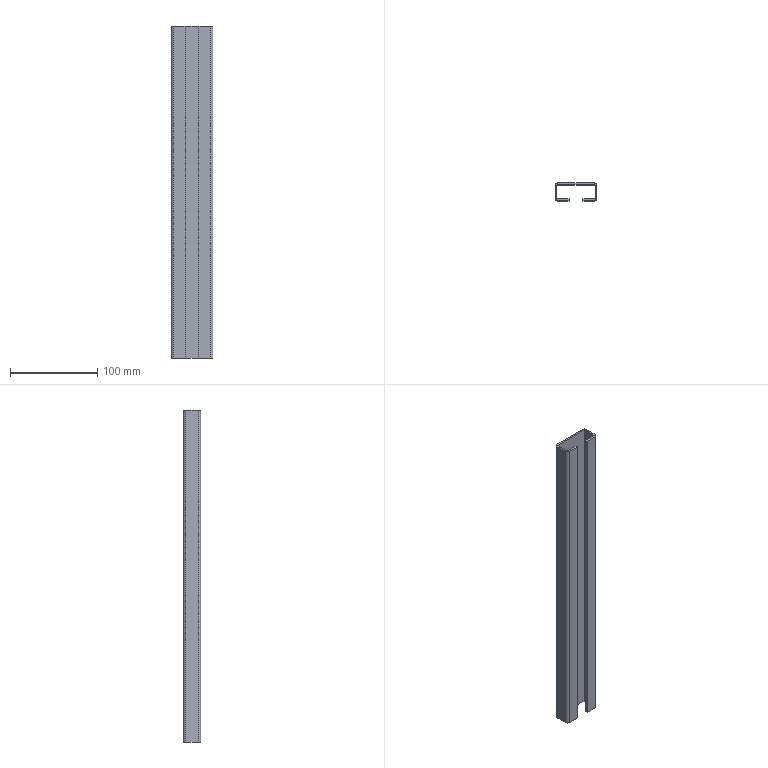Part | SolidWorks | features FlatPattern 1, SMBaseFlange 1, SheetMetal 1 | 1 solid | 38 faces | box 48 x 20 x 380 mm | volume 82510 mm3 | plane 30 | cylinder 8 | commonest cylinder face diameters 2 x4 6 x4
STEP:
#1=CARTESIAN_POINT('',(-24.,-17.,190.));
#2=VERTEX_POINT('',#1);
#3=CARTESIAN_POINT('',(-22.,-17.,190.));
#4=VERTEX_POINT('',#3);
#5=CARTESIAN_POINT('',(-24.,-17.,190.));
#6=DIRECTION('',(1.,0.,0.));
#7=VECTOR('',#6,1000.);
#8=LINE('',#5,#7);
#9=EDGE_CURVE('',#2,#4,#8,.T.);
#10=ORIENTED_EDGE('',*,*,#9,.F.);
#11=CARTESIAN_POINT('',(-21.,-20.,190.));
#12=VERTEX_POINT('',#11);
#13=CARTESIAN_POINT('',(-21.,-17.,190.));
#14=DIRECTION('',(0.,0.,-1.));
#15=DIRECTION('',(1.,0.,0.));
#16=AXIS2_PLACEMENT_3D('',#13,#14,#15);
#17=CIRCLE('',#16,3.);
#18=EDGE_CURVE('',#12,#2,#17,.T.);
#19=ORIENTED_EDGE('',*,*,#18,.F.);
#20=CARTESIAN_POINT('',(-21.,-18.,190.));
#21=VERTEX_POINT('',#20);
#22=CARTESIAN_POINT('',(-21.,-18.,190.));
#23=DIRECTION('',(0.,-1.,0.));
#24=VECTOR('',#23,1000.);
#25=LINE('',#22,#24);
#26=EDGE_CURVE('',#21,#12,#25,.T.);
#27=ORIENTED_EDGE('',*,*,#26,.F.);
#28=CARTESIAN_POINT('',(-21.,-17.,190.));
#29=DIRECTION('',(0.,0.,-1.));
#30=DIRECTION('',(1.,0.,0.));
#31=AXIS2_PLACEMENT_3D('',#28,#29,#30);
#32=CIRCLE('',#31,1.);
#33=EDGE_CURVE('',#21,#4,#32,.T.);
#34=ORIENTED_EDGE('',*,*,#33,.T.);
#35=EDGE_LOOP('',(#10,#19,#27,#34));
#36=FACE_OUTER_BOUND('',#35,.T.);
#37=CARTESIAN_POINT('',(-24.,-17.,190.));
#38=DIRECTION('',(0.,0.,1.));
#39=DIRECTION('',(1.,0.,0.));
#40=AXIS2_PLACEMENT_3D('',#37,#38,#39);
#41=PLANE('',#40);
#42=ADVANCED_FACE('',(#36),#41,.T.);
#43=CARTESIAN_POINT('',(-24.,-3.,190.));
#44=VERTEX_POINT('',#43);
#45=CARTESIAN_POINT('',(-24.,-20.,190.));
#46=DIRECTION('',(0.,1.,0.));
#47=VECTOR('',#46,1000.);
#48=LINE('',#45,#47);
#49=EDGE_CURVE('',#2,#44,#48,.T.);
#50=ORIENTED_EDGE('',*,*,#49,.F.);
#51=ORIENTED_EDGE('',*,*,#9,.T.);
#52=CARTESIAN_POINT('',(-22.,-3.,190.));
#53=VERTEX_POINT('',#52);
#54=CARTESIAN_POINT('',(-22.,-20.,190.));
#55=DIRECTION('',(0.,1.,0.));
#56=VECTOR('',#55,1000.);
#57=LINE('',#54,#56);
#58=EDGE_CURVE('',#4,#53,#57,.T.);
#59=ORIENTED_EDGE('',*,*,#58,.T.);
#60=CARTESIAN_POINT('',(-22.,-3.,190.));
#61=DIRECTION('',(-1.,0.,0.));
#62=VECTOR('',#61,1000.);
#63=LINE('',#60,#62);
#64=EDGE_CURVE('',#53,#44,#63,.T.);
#65=ORIENTED_EDGE('',*,*,#64,.T.);
#66=EDGE_LOOP('',(#50,#51,#59,#65));
#67=FACE_OUTER_BOUND('',#66,.T.);
#68=CARTESIAN_POINT('',(-21.,-18.,190.));
#69=DIRECTION('',(0.,0.,1.));
#70=DIRECTION('',(1.,0.,0.));
#71=AXIS2_PLACEMENT_3D('',#68,#69,#70);
#72=PLANE('',#71);
#73=ADVANCED_FACE('',(#67),#72,.T.);
#74=CARTESIAN_POINT('',(-21.,-20.,-190.));
#75=VERTEX_POINT('',#74);
#76=CARTESIAN_POINT('',(-21.,-18.,-190.));
#77=VERTEX_POINT('',#76);
#78=CARTESIAN_POINT('',(-21.,-20.,-190.));
#79=DIRECTION('',(0.,1.,0.));
#80=VECTOR('',#79,1000.);
#81=LINE('',#78,#80);
#82=EDGE_CURVE('',#75,#77,#81,.T.);
#83=ORIENTED_EDGE('',*,*,#82,.F.);
#84=CARTESIAN_POINT('',(-24.,-17.,-190.));
#85=VERTEX_POINT('',#84);
#86=CARTESIAN_POINT('',(-21.,-17.,-190.));
#87=DIRECTION('',(0.,0.,-1.));
#88=DIRECTION('',(1.,0.,0.));
#89=AXIS2_PLACEMENT_3D('',#86,#87,#88);
#90=CIRCLE('',#89,3.);
#91=EDGE_CURVE('',#75,#85,#90,.T.);
#92=ORIENTED_EDGE('',*,*,#91,.T.);
#93=CARTESIAN_POINT('',(-22.,-17.,-190.));
#94=VERTEX_POINT('',#93);
#95=CARTESIAN_POINT('',(-22.,-17.,-190.));
#96=DIRECTION('',(-1.,0.,0.));
#97=VECTOR('',#96,1000.);
#98=LINE('',#95,#97);
#99=EDGE_CURVE('',#94,#85,#98,.T.);
#100=ORIENTED_EDGE('',*,*,#99,.F.);
#101=CARTESIAN_POINT('',(-21.,-17.,-190.));
#102=DIRECTION('',(0.,0.,-1.));
#103=DIRECTION('',(1.,0.,0.));
#104=AXIS2_PLACEMENT_3D('',#101,#102,#103);
#105=CIRCLE('',#104,1.);
#106=EDGE_CURVE('',#77,#94,#105,.T.);
#107=ORIENTED_EDGE('',*,*,#106,.F.);
#108=EDGE_LOOP('',(#83,#92,#100,#107));
#109=FACE_OUTER_BOUND('',#108,.T.);
#110=CARTESIAN_POINT('',(-21.,-20.,-190.));
#111=DIRECTION('',(0.,0.,-1.));
#112=DIRECTION('',(-1.,0.,0.));
#113=AXIS2_PLACEMENT_3D('',#110,#111,#112);
#114=PLANE('',#113);
#115=ADVANCED_FACE('',(#109),#114,.T.);
#116=CARTESIAN_POINT('',(-8.,-20.,-190.));
#117=VERTEX_POINT('',#116);
#118=CARTESIAN_POINT('',(-8.,-20.,-190.));
#119=DIRECTION('',(-1.,0.,0.));
#120=VECTOR('',#119,1000.);
#121=LINE('',#118,#120);
#122=EDGE_CURVE('',#117,#75,#121,.T.);
#123=ORIENTED_EDGE('',*,*,#122,.T.);
#124=ORIENTED_EDGE('',*,*,#82,.T.);
#125=CARTESIAN_POINT('',(-8.,-18.,-190.));
#126=VERTEX_POINT('',#125);
#127=CARTESIAN_POINT('',(-8.,-18.,-190.));
#128=DIRECTION('',(-1.,0.,0.));
#129=VECTOR('',#128,1000.);
#130=LINE('',#127,#129);
#131=EDGE_CURVE('',#126,#77,#130,.T.);
#132=ORIENTED_EDGE('',*,*,#131,.F.);
#133=CARTESIAN_POINT('',(-8.,-18.,-190.));
#134=DIRECTION('',(0.,-1.,0.));
#135=VECTOR('',#134,1000.);
#136=LINE('',#133,#135);
#137=EDGE_CURVE('',#126,#117,#136,.T.);
#138=ORIENTED_EDGE('',*,*,#137,.T.);
#139=EDGE_LOOP('',(#123,#124,#132,#138));
#140=FACE_OUTER_BOUND('',#139,.T.);
#141=CARTESIAN_POINT('',(-22.,-17.,-190.));
#142=DIRECTION('',(0.,0.,-1.));
#143=DIRECTION('',(-1.,0.,0.));
#144=AXIS2_PLACEMENT_3D('',#141,#142,#143);
#145=PLANE('',#144);
#146=ADVANCED_FACE('',(#140),#145,.T.);
#147=CARTESIAN_POINT('',(-21.,0.,190.));
#148=VERTEX_POINT('',#147);
#149=CARTESIAN_POINT('',(-21.,-2.,190.));
#150=VERTEX_POINT('',#149);
#151=CARTESIAN_POINT('',(-21.,0.,190.));
#152=DIRECTION('',(0.,-1.,0.));
#153=VECTOR('',#152,1000.);
#154=LINE('',#151,#153);
#155=EDGE_CURVE('',#148,#150,#154,.T.);
#156=ORIENTED_EDGE('',*,*,#155,.F.);
#157=CARTESIAN_POINT('',(-21.,-3.,190.));
#158=DIRECTION('',(0.,0.,-1.));
#159=DIRECTION('',(1.,0.,0.));
#160=AXIS2_PLACEMENT_3D('',#157,#158,#159);
#161=CIRCLE('',#160,3.);
#162=EDGE_CURVE('',#44,#148,#161,.T.);
#163=ORIENTED_EDGE('',*,*,#162,.F.);
#164=ORIENTED_EDGE('',*,*,#64,.F.);
#165=CARTESIAN_POINT('',(-21.,-3.,190.));
#166=DIRECTION('',(0.,0.,-1.));
#167=DIRECTION('',(1.,0.,0.));
#168=AXIS2_PLACEMENT_3D('',#165,#166,#167);
#169=CIRCLE('',#168,1.);
#170=EDGE_CURVE('',#53,#150,#169,.T.);
#171=ORIENTED_EDGE('',*,*,#170,.T.);
#172=EDGE_LOOP('',(#156,#163,#164,#171));
#173=FACE_OUTER_BOUND('',#172,.T.);
#174=CARTESIAN_POINT('',(-21.,0.,190.));
#175=DIRECTION('',(0.,0.,1.));
#176=DIRECTION('',(1.,0.,0.));
#177=AXIS2_PLACEMENT_3D('',#174,#175,#176);
#178=PLANE('',#177);
#179=ADVANCED_FACE('',(#173),#178,.T.);
#180=CARTESIAN_POINT('',(21.,0.,190.));
#181=VERTEX_POINT('',#180);
#182=CARTESIAN_POINT('',(-24.,0.,190.));
#183=DIRECTION('',(1.,0.,0.));
#184=VECTOR('',#183,1000.);
#185=LINE('',#182,#184);
#186=EDGE_CURVE('',#148,#181,#185,.T.);
#187=ORIENTED_EDGE('',*,*,#186,.F.);
#188=ORIENTED_EDGE('',*,*,#155,.T.);
#189=CARTESIAN_POINT('',(21.,-2.,190.));
#190=VERTEX_POINT('',#189);
#191=CARTESIAN_POINT('',(-24.,-2.,190.));
#192=DIRECTION('',(1.,0.,0.));
#193=VECTOR('',#192,1000.);
#194=LINE('',#191,#193);
#195=EDGE_CURVE('',#150,#190,#194,.T.);
#196=ORIENTED_EDGE('',*,*,#195,.T.);
#197=CARTESIAN_POINT('',(21.,-2.,190.));
#198=DIRECTION('',(0.,1.,0.));
#199=VECTOR('',#198,1000.);
#200=LINE('',#197,#199);
#201=EDGE_CURVE('',#190,#181,#200,.T.);
#202=ORIENTED_EDGE('',*,*,#201,.T.);
#203=EDGE_LOOP('',(#187,#188,#196,#202));
#204=FACE_OUTER_BOUND('',#203,.T.);
#205=CARTESIAN_POINT('',(-22.,-3.,190.));
#206=DIRECTION('',(0.,0.,1.));
#207=DIRECTION('',(1.,0.,0.));
#208=AXIS2_PLACEMENT_3D('',#205,#206,#207);
#209=PLANE('',#208);
#210=ADVANCED_FACE('',(#204),#209,.T.);
#211=CARTESIAN_POINT('',(-24.,-3.,-190.));
#212=VERTEX_POINT('',#211);
#213=CARTESIAN_POINT('',(-22.,-3.,-190.));
#214=VERTEX_POINT('',#213);
#215=CARTESIAN_POINT('',(-24.,-3.,-190.));
#216=DIRECTION('',(1.,0.,0.));
#217=VECTOR('',#216,1000.);
#218=LINE('',#215,#217);
#219=EDGE_CURVE('',#212,#214,#218,.T.);
#220=ORIENTED_EDGE('',*,*,#219,.F.);
#221=CARTESIAN_POINT('',(-21.,0.,-190.));
#222=VERTEX_POINT('',#221);
#223=CARTESIAN_POINT('',(-21.,-3.,-190.));
#224=DIRECTION('',(0.,0.,-1.));
#225=DIRECTION('',(1.,0.,0.));
#226=AXIS2_PLACEMENT_3D('',#223,#224,#225);
#227=CIRCLE('',#226,3.);
#228=EDGE_CURVE('',#212,#222,#227,.T.);
#229=ORIENTED_EDGE('',*,*,#228,.T.);
#230=CARTESIAN_POINT('',(-21.,-2.,-190.));
#231=VERTEX_POINT('',#230);
#232=CARTESIAN_POINT('',(-21.,-2.,-190.));
#233=DIRECTION('',(0.,1.,0.));
#234=VECTOR('',#233,1000.);
#235=LINE('',#232,#234);
#236=EDGE_CURVE('',#231,#222,#235,.T.);
#237=ORIENTED_EDGE('',*,*,#236,.F.);
#238=CARTESIAN_POINT('',(-21.,-3.,-190.));
#239=DIRECTION('',(0.,0.,-1.));
#240=DIRECTION('',(1.,0.,0.));
#241=AXIS2_PLACEMENT_3D('',#238,#239,#240);
#242=CIRCLE('',#241,1.);
#243=EDGE_CURVE('',#214,#231,#242,.T.);
#244=ORIENTED_EDGE('',*,*,#243,.F.);
#245=EDGE_LOOP('',(#220,#229,#237,#244));
#246=FACE_OUTER_BOUND('',#245,.T.);
#247=CARTESIAN_POINT('',(-24.,-3.,-190.));
#248=DIRECTION('',(0.,0.,-1.));
#249=DIRECTION('',(-1.,0.,0.));
#250=AXIS2_PLACEMENT_3D('',#247,#248,#249);
#251=PLANE('',#250);
#252=ADVANCED_FACE('',(#246),#251,.T.);
#253=CARTESIAN_POINT('',(-24.,-20.,-190.));
#254=DIRECTION('',(0.,1.,0.));
#255=VECTOR('',#254,1000.);
#256=LINE('',#253,#255);
#257=EDGE_CURVE('',#85,#212,#256,.T.);
#258=ORIENTED_EDGE('',*,*,#257,.T.);
#259=ORIENTED_EDGE('',*,*,#219,.T.);
#260=CARTESIAN_POINT('',(-22.,-20.,-190.));
#261=DIRECTION('',(0.,1.,0.));
#262=VECTOR('',#261,1000.);
#263=LINE('',#260,#262);
#264=EDGE_CURVE('',#94,#214,#263,.T.);
#265=ORIENTED_EDGE('',*,*,#264,.F.);
#266=ORIENTED_EDGE('',*,*,#99,.T.);
#267=EDGE_LOOP('',(#258,#259,#265,#266));
#268=FACE_OUTER_BOUND('',#267,.T.);
#269=CARTESIAN_POINT('',(-21.,-2.,-190.));
#270=DIRECTION('',(0.,0.,-1.));
#271=DIRECTION('',(-1.,0.,0.));
#272=AXIS2_PLACEMENT_3D('',#269,#270,#271);
#273=PLANE('',#272);
#274=ADVANCED_FACE('',(#268),#273,.T.);
#275=CARTESIAN_POINT('',(24.,-3.,190.));
#276=VERTEX_POINT('',#275);
#277=CARTESIAN_POINT('',(22.,-3.,190.));
#278=VERTEX_POINT('',#277);
#279=CARTESIAN_POINT('',(24.,-3.,190.));
#280=DIRECTION('',(-1.,0.,0.));
#281=VECTOR('',#280,1000.);
#282=LINE('',#279,#281);
#283=EDGE_CURVE('',#276,#278,#282,.T.);
#284=ORIENTED_EDGE('',*,*,#283,.F.);
#285=CARTESIAN_POINT('',(21.,-3.,190.));
#286=DIRECTION('',(0.,0.,-1.));
#287=DIRECTION('',(1.,0.,0.));
#288=AXIS2_PLACEMENT_3D('',#285,#286,#287);
#289=CIRCLE('',#288,3.);
#290=EDGE_CURVE('',#181,#276,#289,.T.);
#291=ORIENTED_EDGE('',*,*,#290,.F.);
#292=ORIENTED_EDGE('',*,*,#201,.F.);
#293=CARTESIAN_POINT('',(21.,-3.,190.));
#294=DIRECTION('',(0.,0.,-1.));
#295=DIRECTION('',(1.,0.,0.));
#296=AXIS2_PLACEMENT_3D('',#293,#294,#295);
#297=CIRCLE('',#296,1.);
#298=EDGE_CURVE('',#190,#278,#297,.T.);
#299=ORIENTED_EDGE('',*,*,#298,.T.);
#300=EDGE_LOOP('',(#284,#291,#292,#299));
#301=FACE_OUTER_BOUND('',#300,.T.);
#302=CARTESIAN_POINT('',(24.,-3.,190.));
#303=DIRECTION('',(0.,0.,1.));
#304=DIRECTION('',(1.,0.,0.));
#305=AXIS2_PLACEMENT_3D('',#302,#303,#304);
#306=PLANE('',#305);
#307=ADVANCED_FACE('',(#301),#306,.T.);
#308=CARTESIAN_POINT('',(24.,-17.,190.));
#309=VERTEX_POINT('',#308);
#310=CARTESIAN_POINT('',(24.,0.,190.));
#311=DIRECTION('',(0.,-1.,0.));
#312=VECTOR('',#311,1000.);
#313=LINE('',#310,#312);
#314=EDGE_CURVE('',#276,#309,#313,.T.);
#315=ORIENTED_EDGE('',*,*,#314,.F.);
#316=ORIENTED_EDGE('',*,*,#283,.T.);
#317=CARTESIAN_POINT('',(22.,-17.,190.));
#318=VERTEX_POINT('',#317);
#319=CARTESIAN_POINT('',(22.,0.,190.));
#320=DIRECTION('',(0.,-1.,0.));
#321=VECTOR('',#320,1000.);
#322=LINE('',#319,#321);
#323=EDGE_CURVE('',#278,#318,#322,.T.);
#324=ORIENTED_EDGE('',*,*,#323,.T.);
#325=CARTESIAN_POINT('',(22.,-17.,190.));
#326=DIRECTION('',(1.,0.,0.));
#327=VECTOR('',#326,1000.);
#328=LINE('',#325,#327);
#329=EDGE_CURVE('',#318,#309,#328,.T.);
#330=ORIENTED_EDGE('',*,*,#329,.T.);
#331=EDGE_LOOP('',(#315,#316,#324,#330));
#332=FACE_OUTER_BOUND('',#331,.T.);
#333=CARTESIAN_POINT('',(21.,-2.,190.));
#334=DIRECTION('',(0.,0.,1.));
#335=DIRECTION('',(1.,0.,0.));
#336=AXIS2_PLACEMENT_3D('',#333,#334,#335);
#337=PLANE('',#336);
#338=ADVANCED_FACE('',(#332),#337,.T.);
#339=CARTESIAN_POINT('',(21.,0.,-190.));
#340=VERTEX_POINT('',#339);
#341=CARTESIAN_POINT('',(21.,-2.,-190.));
#342=VERTEX_POINT('',#341);
#343=CARTESIAN_POINT('',(21.,0.,-190.));
#344=DIRECTION('',(0.,-1.,0.));
#345=VECTOR('',#344,1000.);
#346=LINE('',#343,#345);
#347=EDGE_CURVE('',#340,#342,#346,.T.);
#348=ORIENTED_EDGE('',*,*,#347,.F.);
#349=CARTESIAN_POINT('',(24.,-3.,-190.));
#350=VERTEX_POINT('',#349);
#351=CARTESIAN_POINT('',(21.,-3.,-190.));
#352=DIRECTION('',(0.,0.,-1.));
#353=DIRECTION('',(1.,0.,0.));
#354=AXIS2_PLACEMENT_3D('',#351,#352,#353);
#355=CIRCLE('',#354,3.);
#356=EDGE_CURVE('',#340,#350,#355,.T.);
#357=ORIENTED_EDGE('',*,*,#356,.T.);
#358=CARTESIAN_POINT('',(22.,-3.,-190.));
#359=VERTEX_POINT('',#358);
#360=CARTESIAN_POINT('',(22.,-3.,-190.));
#361=DIRECTION('',(1.,0.,0.));
#362=VECTOR('',#361,1000.);
#363=LINE('',#360,#362);
#364=EDGE_CURVE('',#359,#350,#363,.T.);
#365=ORIENTED_EDGE('',*,*,#364,.F.);
#366=CARTESIAN_POINT('',(21.,-3.,-190.));
#367=DIRECTION('',(0.,0.,-1.));
#368=DIRECTION('',(1.,0.,0.));
#369=AXIS2_PLACEMENT_3D('',#366,#367,#368);
#370=CIRCLE('',#369,1.);
#371=EDGE_CURVE('',#342,#359,#370,.T.);
#372=ORIENTED_EDGE('',*,*,#371,.F.);
#373=EDGE_LOOP('',(#348,#357,#365,#372));
#374=FACE_OUTER_BOUND('',#373,.T.);
#375=CARTESIAN_POINT('',(21.,0.,-190.));
#376=DIRECTION('',(0.,0.,-1.));
#377=DIRECTION('',(-1.,0.,0.));
#378=AXIS2_PLACEMENT_3D('',#375,#376,#377);
#379=PLANE('',#378);
#380=ADVANCED_FACE('',(#374),#379,.T.);
#381=CARTESIAN_POINT('',(-24.,0.,-190.));
#382=DIRECTION('',(1.,0.,0.));
#383=VECTOR('',#382,1000.);
#384=LINE('',#381,#383);
#385=EDGE_CURVE('',#222,#340,#384,.T.);
#386=ORIENTED_EDGE('',*,*,#385,.T.);
#387=ORIENTED_EDGE('',*,*,#347,.T.);
#388=CARTESIAN_POINT('',(-24.,-2.,-190.));
#389=DIRECTION('',(1.,0.,0.));
#390=VECTOR('',#389,1000.);
#391=LINE('',#388,#390);
#392=EDGE_CURVE('',#231,#342,#391,.T.);
#393=ORIENTED_EDGE('',*,*,#392,.F.);
#394=ORIENTED_EDGE('',*,*,#236,.T.);
#395=EDGE_LOOP('',(#386,#387,#393,#394));
#396=FACE_OUTER_BOUND('',#395,.T.);
#397=CARTESIAN_POINT('',(22.,-3.,-190.));
#398=DIRECTION('',(0.,0.,-1.));
#399=DIRECTION('',(-1.,0.,0.));
#400=AXIS2_PLACEMENT_3D('',#397,#398,#399);
#401=PLANE('',#400);
#402=ADVANCED_FACE('',(#396),#401,.T.);
#403=CARTESIAN_POINT('',(21.,-20.,190.));
#404=VERTEX_POINT('',#403);
#405=CARTESIAN_POINT('',(21.,-18.,190.));
#406=VERTEX_POINT('',#405);
#407=CARTESIAN_POINT('',(21.,-20.,190.));
#408=DIRECTION('',(0.,1.,0.));
#409=VECTOR('',#408,1000.);
#410=LINE('',#407,#409);
#411=EDGE_CURVE('',#404,#406,#410,.T.);
#412=ORIENTED_EDGE('',*,*,#411,.F.);
#413=CARTESIAN_POINT('',(21.,-17.,190.));
#414=DIRECTION('',(0.,0.,-1.));
#415=DIRECTION('',(1.,0.,0.));
#416=AXIS2_PLACEMENT_3D('',#413,#414,#415);
#417=CIRCLE('',#416,3.);
#418=EDGE_CURVE('',#309,#404,#417,.T.);
#419=ORIENTED_EDGE('',*,*,#418,.F.);
#420=ORIENTED_EDGE('',*,*,#329,.F.);
#421=CARTESIAN_POINT('',(21.,-17.,190.));
#422=DIRECTION('',(0.,0.,-1.));
#423=DIRECTION('',(1.,0.,0.));
#424=AXIS2_PLACEMENT_3D('',#421,#422,#423);
#425=CIRCLE('',#424,1.);
#426=EDGE_CURVE('',#318,#406,#425,.T.);
#427=ORIENTED_EDGE('',*,*,#426,.T.);
#428=EDGE_LOOP('',(#412,#419,#420,#427));
#429=FACE_OUTER_BOUND('',#428,.T.);
#430=CARTESIAN_POINT('',(21.,-20.,190.));
#431=DIRECTION('',(0.,0.,1.));
#432=DIRECTION('',(1.,0.,0.));
#433=AXIS2_PLACEMENT_3D('',#430,#431,#432);
#434=PLANE('',#433);
#435=ADVANCED_FACE('',(#429),#434,.T.);
#436=CARTESIAN_POINT('',(8.,-20.,190.));
#437=VERTEX_POINT('',#436);
#438=CARTESIAN_POINT('',(24.,-20.,190.));
#439=DIRECTION('',(-1.,0.,0.));
#440=VECTOR('',#439,1000.);
#441=LINE('',#438,#440);
#442=EDGE_CURVE('',#404,#437,#441,.T.);
#443=ORIENTED_EDGE('',*,*,#442,.F.);
#444=ORIENTED_EDGE('',*,*,#411,.T.);
#445=CARTESIAN_POINT('',(8.,-18.,190.));
#446=VERTEX_POINT('',#445);
#447=CARTESIAN_POINT('',(24.,-18.,190.));
#448=DIRECTION('',(-1.,0.,0.));
#449=VECTOR('',#448,1000.);
#450=LINE('',#447,#449);
#451=EDGE_CURVE('',#406,#446,#450,.T.);
#452=ORIENTED_EDGE('',*,*,#451,.T.);
#453=CARTESIAN_POINT('',(8.,-20.,190.));
#454=DIRECTION('',(0.,1.,0.));
#455=VECTOR('',#454,1000.);
#456=LINE('',#453,#455);
#457=EDGE_CURVE('',#437,#446,#456,.T.);
#458=ORIENTED_EDGE('',*,*,#457,.F.);
#459=EDGE_LOOP('',(#443,#444,#452,#458));
#460=FACE_OUTER_BOUND('',#459,.T.);
#461=CARTESIAN_POINT('',(22.,-17.,190.));
#462=DIRECTION('',(0.,0.,1.));
#463=DIRECTION('',(1.,0.,0.));
#464=AXIS2_PLACEMENT_3D('',#461,#462,#463);
#465=PLANE('',#464);
#466=ADVANCED_FACE('',(#460),#465,.T.);
#467=CARTESIAN_POINT('',(24.,-17.,-190.));
#468=VERTEX_POINT('',#467);
#469=CARTESIAN_POINT('',(22.,-17.,-190.));
#470=VERTEX_POINT('',#469);
#471=CARTESIAN_POINT('',(24.,-17.,-190.));
#472=DIRECTION('',(-1.,0.,0.));
#473=VECTOR('',#472,1000.);
#474=LINE('',#471,#473);
#475=EDGE_CURVE('',#468,#470,#474,.T.);
#476=ORIENTED_EDGE('',*,*,#475,.F.);
#477=CARTESIAN_POINT('',(21.,-20.,-190.));
#478=VERTEX_POINT('',#477);
#479=CARTESIAN_POINT('',(21.,-17.,-190.));
#480=DIRECTION('',(0.,0.,-1.));
#481=DIRECTION('',(1.,0.,0.));
#482=AXIS2_PLACEMENT_3D('',#479,#480,#481);
#483=CIRCLE('',#482,3.);
#484=EDGE_CURVE('',#468,#478,#483,.T.);
#485=ORIENTED_EDGE('',*,*,#484,.T.);
#486=CARTESIAN_POINT('',(21.,-18.,-190.));
#487=VERTEX_POINT('',#486);
#488=CARTESIAN_POINT('',(21.,-18.,-190.));
#489=DIRECTION('',(0.,-1.,0.));
#490=VECTOR('',#489,1000.);
#491=LINE('',#488,#490);
#492=EDGE_CURVE('',#487,#478,#491,.T.);
#493=ORIENTED_EDGE('',*,*,#492,.F.);
#494=CARTESIAN_POINT('',(21.,-17.,-190.));
#495=DIRECTION('',(0.,0.,-1.));
#496=DIRECTION('',(1.,0.,0.));
#497=AXIS2_PLACEMENT_3D('',#494,#495,#496);
#498=CIRCLE('',#497,1.);
#499=EDGE_CURVE('',#470,#487,#498,.T.);
#500=ORIENTED_EDGE('',*,*,#499,.F.);
#501=EDGE_LOOP('',(#476,#485,#493,#500));
#502=FACE_OUTER_BOUND('',#501,.T.);
#503=CARTESIAN_POINT('',(24.,-17.,-190.));
#504=DIRECTION('',(0.,0.,-1.));
#505=DIRECTION('',(-1.,0.,0.));
#506=AXIS2_PLACEMENT_3D('',#503,#504,#505);
#507=PLANE('',#506);
#508=ADVANCED_FACE('',(#502),#507,.T.);
#509=CARTESIAN_POINT('',(24.,0.,-190.));
#510=DIRECTION('',(0.,-1.,0.));
#511=VECTOR('',#510,1000.);
#512=LINE('',#509,#511);
#513=EDGE_CURVE('',#350,#468,#512,.T.);
#514=ORIENTED_EDGE('',*,*,#513,.T.);
#515=ORIENTED_EDGE('',*,*,#475,.T.);
#516=CARTESIAN_POINT('',(22.,0.,-190.));
#517=DIRECTION('',(0.,-1.,0.));
#518=VECTOR('',#517,1000.);
#519=LINE('',#516,#518);
#520=EDGE_CURVE('',#359,#470,#519,.T.);
#521=ORIENTED_EDGE('',*,*,#520,.F.);
#522=ORIENTED_EDGE('',*,*,#364,.T.);
#523=EDGE_LOOP('',(#514,#515,#521,#522));
#524=FACE_OUTER_BOUND('',#523,.T.);
#525=CARTESIAN_POINT('',(21.,-18.,-190.));
#526=DIRECTION('',(0.,0.,-1.));
#527=DIRECTION('',(-1.,0.,0.));
#528=AXIS2_PLACEMENT_3D('',#525,#526,#527);
#529=PLANE('',#528);
#530=ADVANCED_FACE('',(#524),#529,.T.);
#531=CARTESIAN_POINT('',(8.,-18.,-190.));
#532=VERTEX_POINT('',#531);
#533=CARTESIAN_POINT('',(24.,-18.,-190.));
#534=DIRECTION('',(-1.,0.,0.));
#535=VECTOR('',#534,1000.);
#536=LINE('',#533,#535);
#537=EDGE_CURVE('',#487,#532,#536,.T.);
#538=ORIENTED_EDGE('',*,*,#537,.T.);
#539=CARTESIAN_POINT('',(8.,-18.,190.));
#540=DIRECTION('',(0.,0.,-1.));
#541=VECTOR('',#540,1000.);
#542=LINE('',#539,#541);
#543=EDGE_CURVE('',#446,#532,#542,.T.);
#544=ORIENTED_EDGE('',*,*,#543,.F.);
#545=ORIENTED_EDGE('',*,*,#451,.F.);
#546=CARTESIAN_POINT('',(21.,-18.,190.));
#547=DIRECTION('',(0.,0.,-1.));
#548=VECTOR('',#547,1000.);
#549=LINE('',#546,#548);
#550=EDGE_CURVE('',#406,#487,#549,.T.);
#551=ORIENTED_EDGE('',*,*,#550,.T.);
#552=EDGE_LOOP('',(#538,#544,#545,#551));
#553=FACE_OUTER_BOUND('',#552,.T.);
#554=CARTESIAN_POINT('',(24.,-18.,190.));
#555=DIRECTION('',(0.,-1.,0.));
#556=DIRECTION('',(1.,0.,0.));
#557=AXIS2_PLACEMENT_3D('',#554,#555,#556);
#558=PLANE('',#557);
#559=ADVANCED_FACE('',(#553),#558,.F.);
#560=CARTESIAN_POINT('',(8.,-20.,-190.));
#561=VERTEX_POINT('',#560);
#562=CARTESIAN_POINT('',(8.,-20.,-190.));
#563=DIRECTION('',(0.,1.,0.));
#564=VECTOR('',#563,1000.);
#565=LINE('',#562,#564);
#566=EDGE_CURVE('',#561,#532,#565,.T.);
#567=ORIENTED_EDGE('',*,*,#566,.F.);
#568=CARTESIAN_POINT('',(8.,-20.,190.));
#569=DIRECTION('',(0.,0.,-1.));
#570=VECTOR('',#569,1000.);
#571=LINE('',#568,#570);
#572=EDGE_CURVE('',#437,#561,#571,.T.);
#573=ORIENTED_EDGE('',*,*,#572,.F.);
#574=ORIENTED_EDGE('',*,*,#457,.T.);
#575=ORIENTED_EDGE('',*,*,#543,.T.);
#576=EDGE_LOOP('',(#567,#573,#574,#575));
#577=FACE_OUTER_BOUND('',#576,.T.);
#578=CARTESIAN_POINT('',(8.,-20.,190.));
#579=DIRECTION('',(-1.,0.,0.));
#580=DIRECTION('',(0.,0.,1.));
#581=AXIS2_PLACEMENT_3D('',#578,#579,#580);
#582=PLANE('',#581);
#583=ADVANCED_FACE('',(#577),#582,.T.);
#584=CARTESIAN_POINT('',(24.,-20.,-190.));
#585=DIRECTION('',(-1.,0.,0.));
#586=VECTOR('',#585,1000.);
#587=LINE('',#584,#586);
#588=EDGE_CURVE('',#478,#561,#587,.T.);
#589=ORIENTED_EDGE('',*,*,#588,.F.);
#590=CARTESIAN_POINT('',(21.,-20.,190.));
#591=DIRECTION('',(0.,0.,-1.));
#592=VECTOR('',#591,1000.);
#593=LINE('',#590,#592);
#594=EDGE_CURVE('',#404,#478,#593,.T.);
#595=ORIENTED_EDGE('',*,*,#594,.F.);
#596=ORIENTED_EDGE('',*,*,#442,.T.);
#597=ORIENTED_EDGE('',*,*,#572,.T.);
#598=EDGE_LOOP('',(#589,#595,#596,#597));
#599=FACE_OUTER_BOUND('',#598,.T.);
#600=CARTESIAN_POINT('',(24.,-20.,190.));
#601=DIRECTION('',(0.,-1.,0.));
#602=DIRECTION('',(1.,0.,0.));
#603=AXIS2_PLACEMENT_3D('',#600,#601,#602);
#604=PLANE('',#603);
#605=ADVANCED_FACE('',(#599),#604,.T.);
#606=ORIENTED_EDGE('',*,*,#484,.F.);
#607=CARTESIAN_POINT('',(24.,-17.,190.));
#608=DIRECTION('',(0.,0.,-1.));
#609=VECTOR('',#608,1000.);
#610=LINE('',#607,#609);
#611=EDGE_CURVE('',#309,#468,#610,.T.);
#612=ORIENTED_EDGE('',*,*,#611,.F.);
#613=ORIENTED_EDGE('',*,*,#418,.T.);
#614=ORIENTED_EDGE('',*,*,#594,.T.);
#615=EDGE_LOOP('',(#606,#612,#613,#614));
#616=FACE_OUTER_BOUND('',#615,.T.);
#617=CARTESIAN_POINT('',(21.,-17.,190.));
#618=DIRECTION('',(0.,0.,-1.));
#619=DIRECTION('',(-1.,0.,0.));
#620=AXIS2_PLACEMENT_3D('',#617,#618,#619);
#621=CYLINDRICAL_SURFACE('',#620,3.);
#622=ADVANCED_FACE('',(#616),#621,.T.);
#623=ORIENTED_EDGE('',*,*,#513,.F.);
#624=CARTESIAN_POINT('',(24.,-3.,190.));
#625=DIRECTION('',(0.,0.,-1.));
#626=VECTOR('',#625,1000.);
#627=LINE('',#624,#626);
#628=EDGE_CURVE('',#276,#350,#627,.T.);
#629=ORIENTED_EDGE('',*,*,#628,.F.);
#630=ORIENTED_EDGE('',*,*,#314,.T.);
#631=ORIENTED_EDGE('',*,*,#611,.T.);
#632=EDGE_LOOP('',(#623,#629,#630,#631));
#633=FACE_OUTER_BOUND('',#632,.T.);
#634=CARTESIAN_POINT('',(24.,0.,190.));
#635=DIRECTION('',(1.,0.,0.));
#636=DIRECTION('',(0.,0.,-1.));
#637=AXIS2_PLACEMENT_3D('',#634,#635,#636);
#638=PLANE('',#637);
#639=ADVANCED_FACE('',(#633),#638,.T.);
#640=ORIENTED_EDGE('',*,*,#356,.F.);
#641=CARTESIAN_POINT('',(21.,0.,190.));
#642=DIRECTION('',(0.,0.,-1.));
#643=VECTOR('',#642,1000.);
#644=LINE('',#641,#643);
#645=EDGE_CURVE('',#181,#340,#644,.T.);
#646=ORIENTED_EDGE('',*,*,#645,.F.);
#647=ORIENTED_EDGE('',*,*,#290,.T.);
#648=ORIENTED_EDGE('',*,*,#628,.T.);
#649=EDGE_LOOP('',(#640,#646,#647,#648));
#650=FACE_OUTER_BOUND('',#649,.T.);
#651=CARTESIAN_POINT('',(21.,-3.,190.));
#652=DIRECTION('',(0.,0.,-1.));
#653=DIRECTION('',(-1.,0.,0.));
#654=AXIS2_PLACEMENT_3D('',#651,#652,#653);
#655=CYLINDRICAL_SURFACE('',#654,3.);
#656=ADVANCED_FACE('',(#650),#655,.T.);
#657=ORIENTED_EDGE('',*,*,#385,.F.);
#658=CARTESIAN_POINT('',(-21.,0.,190.));
#659=DIRECTION('',(0.,0.,-1.));
#660=VECTOR('',#659,1000.);
#661=LINE('',#658,#660);
#662=EDGE_CURVE('',#148,#222,#661,.T.);
#663=ORIENTED_EDGE('',*,*,#662,.F.);
#664=ORIENTED_EDGE('',*,*,#186,.T.);
#665=ORIENTED_EDGE('',*,*,#645,.T.);
#666=EDGE_LOOP('',(#657,#663,#664,#665));
#667=FACE_OUTER_BOUND('',#666,.T.);
#668=CARTESIAN_POINT('',(-24.,0.,190.));
#669=DIRECTION('',(0.,1.,0.));
#670=DIRECTION('',(0.,0.,1.));
#671=AXIS2_PLACEMENT_3D('',#668,#669,#670);
#672=PLANE('',#671);
#673=ADVANCED_FACE('',(#667),#672,.T.);
#674=ORIENTED_EDGE('',*,*,#228,.F.);
#675=CARTESIAN_POINT('',(-24.,-3.,190.));
#676=DIRECTION('',(0.,0.,-1.));
#677=VECTOR('',#676,1000.);
#678=LINE('',#675,#677);
#679=EDGE_CURVE('',#44,#212,#678,.T.);
#680=ORIENTED_EDGE('',*,*,#679,.F.);
#681=ORIENTED_EDGE('',*,*,#162,.T.);
#682=ORIENTED_EDGE('',*,*,#662,.T.);
#683=EDGE_LOOP('',(#674,#680,#681,#682));
#684=FACE_OUTER_BOUND('',#683,.T.);
#685=CARTESIAN_POINT('',(-21.,-3.,190.));
#686=DIRECTION('',(0.,0.,-1.));
#687=DIRECTION('',(-1.,0.,0.));
#688=AXIS2_PLACEMENT_3D('',#685,#686,#687);
#689=CYLINDRICAL_SURFACE('',#688,3.);
#690=ADVANCED_FACE('',(#684),#689,.T.);
#691=ORIENTED_EDGE('',*,*,#257,.F.);
#692=CARTESIAN_POINT('',(-24.,-17.,190.));
#693=DIRECTION('',(0.,0.,-1.));
#694=VECTOR('',#693,1000.);
#695=LINE('',#692,#694);
#696=EDGE_CURVE('',#2,#85,#695,.T.);
#697=ORIENTED_EDGE('',*,*,#696,.F.);
#698=ORIENTED_EDGE('',*,*,#49,.T.);
#699=ORIENTED_EDGE('',*,*,#679,.T.);
#700=EDGE_LOOP('',(#691,#697,#698,#699));
#701=FACE_OUTER_BOUND('',#700,.T.);
#702=CARTESIAN_POINT('',(-24.,-20.,190.));
#703=DIRECTION('',(-1.,0.,0.));
#704=DIRECTION('',(0.,0.,1.));
#705=AXIS2_PLACEMENT_3D('',#702,#703,#704);
#706=PLANE('',#705);
#707=ADVANCED_FACE('',(#701),#706,.T.);
#708=ORIENTED_EDGE('',*,*,#91,.F.);
#709=CARTESIAN_POINT('',(-21.,-20.,190.));
#710=DIRECTION('',(0.,0.,-1.));
#711=VECTOR('',#710,1000.);
#712=LINE('',#709,#711);
#713=EDGE_CURVE('',#12,#75,#712,.T.);
#714=ORIENTED_EDGE('',*,*,#713,.F.);
#715=ORIENTED_EDGE('',*,*,#18,.T.);
#716=ORIENTED_EDGE('',*,*,#696,.T.);
#717=EDGE_LOOP('',(#708,#714,#715,#716));
#718=FACE_OUTER_BOUND('',#717,.T.);
#719=CARTESIAN_POINT('',(-21.,-17.,190.));
#720=DIRECTION('',(0.,0.,-1.));
#721=DIRECTION('',(-1.,0.,0.));
#722=AXIS2_PLACEMENT_3D('',#719,#720,#721);
#723=CYLINDRICAL_SURFACE('',#722,3.);
#724=ADVANCED_FACE('',(#718),#723,.T.);
#725=ORIENTED_EDGE('',*,*,#122,.F.);
#726=CARTESIAN_POINT('',(-8.,-20.,190.));
#727=VERTEX_POINT('',#726);
#728=CARTESIAN_POINT('',(-8.,-20.,190.));
#729=DIRECTION('',(0.,0.,-1.));
#730=VECTOR('',#729,1000.);
#731=LINE('',#728,#730);
#732=EDGE_CURVE('',#727,#117,#731,.T.);
#733=ORIENTED_EDGE('',*,*,#732,.F.);
#734=CARTESIAN_POINT('',(-8.,-20.,190.));
#735=DIRECTION('',(-1.,0.,0.));
#736=VECTOR('',#735,1000.);
#737=LINE('',#734,#736);
#738=EDGE_CURVE('',#727,#12,#737,.T.);
#739=ORIENTED_EDGE('',*,*,#738,.T.);
#740=ORIENTED_EDGE('',*,*,#713,.T.);
#741=EDGE_LOOP('',(#725,#733,#739,#740));
#742=FACE_OUTER_BOUND('',#741,.T.);
#743=CARTESIAN_POINT('',(-8.,-20.,190.));
#744=DIRECTION('',(0.,-1.,0.));
#745=DIRECTION('',(1.,0.,0.));
#746=AXIS2_PLACEMENT_3D('',#743,#744,#745);
#747=PLANE('',#746);
#748=ADVANCED_FACE('',(#742),#747,.T.);
#749=ORIENTED_EDGE('',*,*,#137,.F.);
#750=CARTESIAN_POINT('',(-8.,-18.,190.));
#751=VERTEX_POINT('',#750);
#752=CARTESIAN_POINT('',(-8.,-18.,190.));
#753=DIRECTION('',(0.,0.,-1.));
#754=VECTOR('',#753,1000.);
#755=LINE('',#752,#754);
#756=EDGE_CURVE('',#751,#126,#755,.T.);
#757=ORIENTED_EDGE('',*,*,#756,.F.);
#758=CARTESIAN_POINT('',(-8.,-18.,190.));
#759=DIRECTION('',(0.,-1.,0.));
#760=VECTOR('',#759,1000.);
#761=LINE('',#758,#760);
#762=EDGE_CURVE('',#751,#727,#761,.T.);
#763=ORIENTED_EDGE('',*,*,#762,.T.);
#764=ORIENTED_EDGE('',*,*,#732,.T.);
#765=EDGE_LOOP('',(#749,#757,#763,#764));
#766=FACE_OUTER_BOUND('',#765,.T.);
#767=CARTESIAN_POINT('',(-8.,-18.,190.));
#768=DIRECTION('',(1.,0.,0.));
#769=DIRECTION('',(0.,0.,-1.));
#770=AXIS2_PLACEMENT_3D('',#767,#768,#769);
#771=PLANE('',#770);
#772=ADVANCED_FACE('',(#766),#771,.T.);
#773=ORIENTED_EDGE('',*,*,#131,.T.);
#774=CARTESIAN_POINT('',(-21.,-18.,190.));
#775=DIRECTION('',(0.,0.,-1.));
#776=VECTOR('',#775,1000.);
#777=LINE('',#774,#776);
#778=EDGE_CURVE('',#21,#77,#777,.T.);
#779=ORIENTED_EDGE('',*,*,#778,.F.);
#780=CARTESIAN_POINT('',(-8.,-18.,190.));
#781=DIRECTION('',(-1.,0.,0.));
#782=VECTOR('',#781,1000.);
#783=LINE('',#780,#782);
#784=EDGE_CURVE('',#751,#21,#783,.T.);
#785=ORIENTED_EDGE('',*,*,#784,.F.);
#786=ORIENTED_EDGE('',*,*,#756,.T.);
#787=EDGE_LOOP('',(#773,#779,#785,#786));
#788=FACE_OUTER_BOUND('',#787,.T.);
#789=CARTESIAN_POINT('',(-8.,-18.,190.));
#790=DIRECTION('',(0.,-1.,0.));
#791=DIRECTION('',(1.,0.,0.));
#792=AXIS2_PLACEMENT_3D('',#789,#790,#791);
#793=PLANE('',#792);
#794=ADVANCED_FACE('',(#788),#793,.F.);
#795=ORIENTED_EDGE('',*,*,#106,.T.);
#796=CARTESIAN_POINT('',(-22.,-17.,190.));
#797=DIRECTION('',(0.,0.,-1.));
#798=VECTOR('',#797,1000.);
#799=LINE('',#796,#798);
#800=EDGE_CURVE('',#4,#94,#799,.T.);
#801=ORIENTED_EDGE('',*,*,#800,.F.);
#802=ORIENTED_EDGE('',*,*,#33,.F.);
#803=ORIENTED_EDGE('',*,*,#778,.T.);
#804=EDGE_LOOP('',(#795,#801,#802,#803));
#805=FACE_OUTER_BOUND('',#804,.T.);
#806=CARTESIAN_POINT('',(-21.,-17.,190.));
#807=DIRECTION('',(0.,0.,-1.));
#808=DIRECTION('',(-1.,0.,0.));
#809=AXIS2_PLACEMENT_3D('',#806,#807,#808);
#810=CYLINDRICAL_SURFACE('',#809,1.);
#811=ADVANCED_FACE('',(#805),#810,.F.);
#812=ORIENTED_EDGE('',*,*,#264,.T.);
#813=CARTESIAN_POINT('',(-22.,-3.,190.));
#814=DIRECTION('',(0.,0.,-1.));
#815=VECTOR('',#814,1000.);
#816=LINE('',#813,#815);
#817=EDGE_CURVE('',#53,#214,#816,.T.);
#818=ORIENTED_EDGE('',*,*,#817,.F.);
#819=ORIENTED_EDGE('',*,*,#58,.F.);
#820=ORIENTED_EDGE('',*,*,#800,.T.);
#821=EDGE_LOOP('',(#812,#818,#819,#820));
#822=FACE_OUTER_BOUND('',#821,.T.);
#823=CARTESIAN_POINT('',(-22.,-20.,190.));
#824=DIRECTION('',(-1.,0.,0.));
#825=DIRECTION('',(0.,0.,1.));
#826=AXIS2_PLACEMENT_3D('',#823,#824,#825);
#827=PLANE('',#826);
#828=ADVANCED_FACE('',(#822),#827,.F.);
#829=ORIENTED_EDGE('',*,*,#243,.T.);
#830=CARTESIAN_POINT('',(-21.,-2.,190.));
#831=DIRECTION('',(0.,0.,-1.));
#832=VECTOR('',#831,1000.);
#833=LINE('',#830,#832);
#834=EDGE_CURVE('',#150,#231,#833,.T.);
#835=ORIENTED_EDGE('',*,*,#834,.F.);
#836=ORIENTED_EDGE('',*,*,#170,.F.);
#837=ORIENTED_EDGE('',*,*,#817,.T.);
#838=EDGE_LOOP('',(#829,#835,#836,#837));
#839=FACE_OUTER_BOUND('',#838,.T.);
#840=CARTESIAN_POINT('',(-21.,-3.,190.));
#841=DIRECTION('',(0.,0.,-1.));
#842=DIRECTION('',(-1.,0.,0.));
#843=AXIS2_PLACEMENT_3D('',#840,#841,#842);
#844=CYLINDRICAL_SURFACE('',#843,1.);
#845=ADVANCED_FACE('',(#839),#844,.F.);
#846=ORIENTED_EDGE('',*,*,#392,.T.);
#847=CARTESIAN_POINT('',(21.,-2.,190.));
#848=DIRECTION('',(0.,0.,-1.));
#849=VECTOR('',#848,1000.);
#850=LINE('',#847,#849);
#851=EDGE_CURVE('',#190,#342,#850,.T.);
#852=ORIENTED_EDGE('',*,*,#851,.F.);
#853=ORIENTED_EDGE('',*,*,#195,.F.);
#854=ORIENTED_EDGE('',*,*,#834,.T.);
#855=EDGE_LOOP('',(#846,#852,#853,#854));
#856=FACE_OUTER_BOUND('',#855,.T.);
#857=CARTESIAN_POINT('',(-24.,-2.,190.));
#858=DIRECTION('',(0.,1.,0.));
#859=DIRECTION('',(0.,0.,1.));
#860=AXIS2_PLACEMENT_3D('',#857,#858,#859);
#861=PLANE('',#860);
#862=ADVANCED_FACE('',(#856),#861,.F.);
#863=ORIENTED_EDGE('',*,*,#371,.T.);
#864=CARTESIAN_POINT('',(22.,-3.,190.));
#865=DIRECTION('',(0.,0.,-1.));
#866=VECTOR('',#865,1000.);
#867=LINE('',#864,#866);
#868=EDGE_CURVE('',#278,#359,#867,.T.);
#869=ORIENTED_EDGE('',*,*,#868,.F.);
#870=ORIENTED_EDGE('',*,*,#298,.F.);
#871=ORIENTED_EDGE('',*,*,#851,.T.);
#872=EDGE_LOOP('',(#863,#869,#870,#871));
#873=FACE_OUTER_BOUND('',#872,.T.);
#874=CARTESIAN_POINT('',(21.,-3.,190.));
#875=DIRECTION('',(0.,0.,-1.));
#876=DIRECTION('',(-1.,0.,0.));
#877=AXIS2_PLACEMENT_3D('',#874,#875,#876);
#878=CYLINDRICAL_SURFACE('',#877,1.);
#879=ADVANCED_FACE('',(#873),#878,.F.);
#880=ORIENTED_EDGE('',*,*,#520,.T.);
#881=CARTESIAN_POINT('',(22.,-17.,190.));
#882=DIRECTION('',(0.,0.,-1.));
#883=VECTOR('',#882,1000.);
#884=LINE('',#881,#883);
#885=EDGE_CURVE('',#318,#470,#884,.T.);
#886=ORIENTED_EDGE('',*,*,#885,.F.);
#887=ORIENTED_EDGE('',*,*,#323,.F.);
#888=ORIENTED_EDGE('',*,*,#868,.T.);
#889=EDGE_LOOP('',(#880,#886,#887,#888));
#890=FACE_OUTER_BOUND('',#889,.T.);
#891=CARTESIAN_POINT('',(22.,0.,190.));
#892=DIRECTION('',(1.,0.,0.));
#893=DIRECTION('',(0.,0.,-1.));
#894=AXIS2_PLACEMENT_3D('',#891,#892,#893);
#895=PLANE('',#894);
#896=ADVANCED_FACE('',(#890),#895,.F.);
#897=ORIENTED_EDGE('',*,*,#499,.T.);
#898=ORIENTED_EDGE('',*,*,#550,.F.);
#899=ORIENTED_EDGE('',*,*,#426,.F.);
#900=ORIENTED_EDGE('',*,*,#885,.T.);
#901=EDGE_LOOP('',(#897,#898,#899,#900));
#902=FACE_OUTER_BOUND('',#901,.T.);
#903=CARTESIAN_POINT('',(21.,-17.,190.));
#904=DIRECTION('',(0.,0.,-1.));
#905=DIRECTION('',(-1.,0.,0.));
#906=AXIS2_PLACEMENT_3D('',#903,#904,#905);
#907=CYLINDRICAL_SURFACE('',#906,1.);
#908=ADVANCED_FACE('',(#902),#907,.F.);
#909=ORIENTED_EDGE('',*,*,#784,.T.);
#910=ORIENTED_EDGE('',*,*,#26,.T.);
#911=ORIENTED_EDGE('',*,*,#738,.F.);
#912=ORIENTED_EDGE('',*,*,#762,.F.);
#913=EDGE_LOOP('',(#909,#910,#911,#912));
#914=FACE_OUTER_BOUND('',#913,.T.);
#915=CARTESIAN_POINT('',(21.,-17.,190.));
#916=DIRECTION('',(0.,0.,1.));
#917=DIRECTION('',(1.,0.,0.));
#918=AXIS2_PLACEMENT_3D('',#915,#916,#917);
#919=PLANE('',#918);
#920=ADVANCED_FACE('',(#914),#919,.T.);
#921=ORIENTED_EDGE('',*,*,#537,.F.);
#922=ORIENTED_EDGE('',*,*,#492,.T.);
#923=ORIENTED_EDGE('',*,*,#588,.T.);
#924=ORIENTED_EDGE('',*,*,#566,.T.);
#925=EDGE_LOOP('',(#921,#922,#923,#924));
#926=FACE_OUTER_BOUND('',#925,.T.);
#927=CARTESIAN_POINT('',(21.,-17.,-190.));
#928=DIRECTION('',(0.,0.,1.));
#929=DIRECTION('',(1.,0.,0.));
#930=AXIS2_PLACEMENT_3D('',#927,#928,#929);
#931=PLANE('',#930);
#932=ADVANCED_FACE('',(#926),#931,.F.);
#933=CLOSED_SHELL('',(#42,#73,#115,#146,#179,#210,#252,#274,#307,#338,#380,#402,#435,#466,#508,#530,#559,#583,#605,#622,#639,#656,#673,#690,#707,#724,#748,#772,#794,#811,#828,#845,#862,#879,#896,#908,#920,#932));
#934=MANIFOLD_SOLID_BREP('',#933);
#935=CARTESIAN_POINT('',(0.,0.,0.));
#936=DIRECTION('',(0.,0.,1.));
#937=DIRECTION('',(1.,0.,0.));
#938=AXIS2_PLACEMENT_3D('',#935,#936,#937);
#939=(LENGTH_UNIT()NAMED_UNIT(*)SI_UNIT(.MILLI.,.METRE.));
#940=UNCERTAINTY_MEASURE_WITH_UNIT(LENGTH_MEASURE(0.00001),#939,'','');
#941=(NAMED_UNIT(*)PLANE_ANGLE_UNIT()SI_UNIT($,.RADIAN.));
#942=(NAMED_UNIT(*)SI_UNIT($,.STERADIAN.)SOLID_ANGLE_UNIT());
#943=(GEOMETRIC_REPRESENTATION_CONTEXT(3)GLOBAL_UNCERTAINTY_ASSIGNED_CONTEXT((#940))GLOBAL_UNIT_ASSIGNED_CONTEXT((#939,#941,#942))REPRESENTATION_CONTEXT('',''));
#944=ADVANCED_BREP_SHAPE_REPRESENTATION('',(#934,#938),#943);